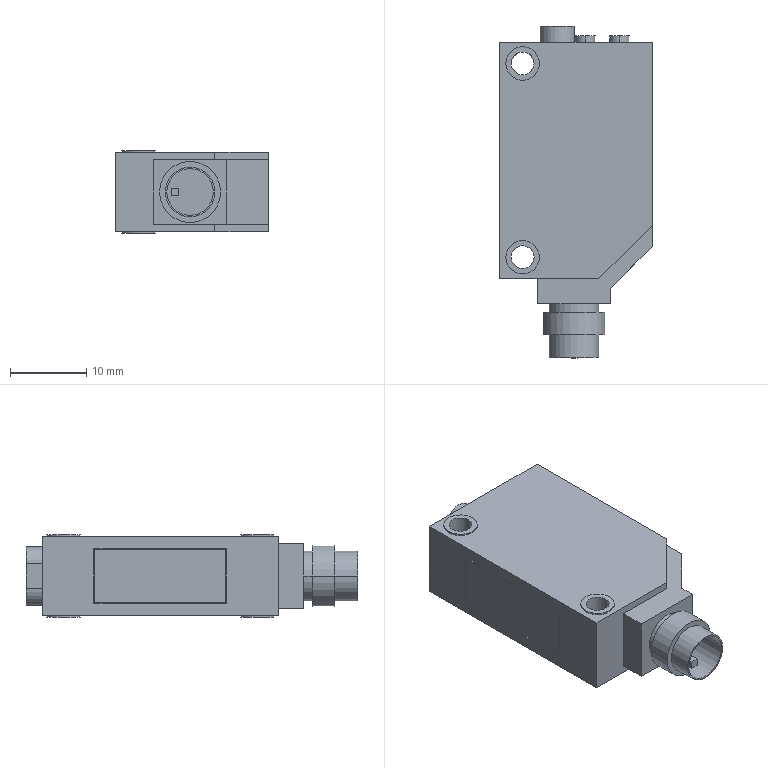Part | STEP file | PN_0045_diffuse photoelectric sensor | 1 solid | 89 faces | box 20 x 43.5 x 10.8 mm | volume 6643 mm3 | plane 62 | cylinder 27 | commonest cylinder face diameters 4.4 x8 2.6 x4 3 x4 6.5 x4 4.5 x3 6.1 x2